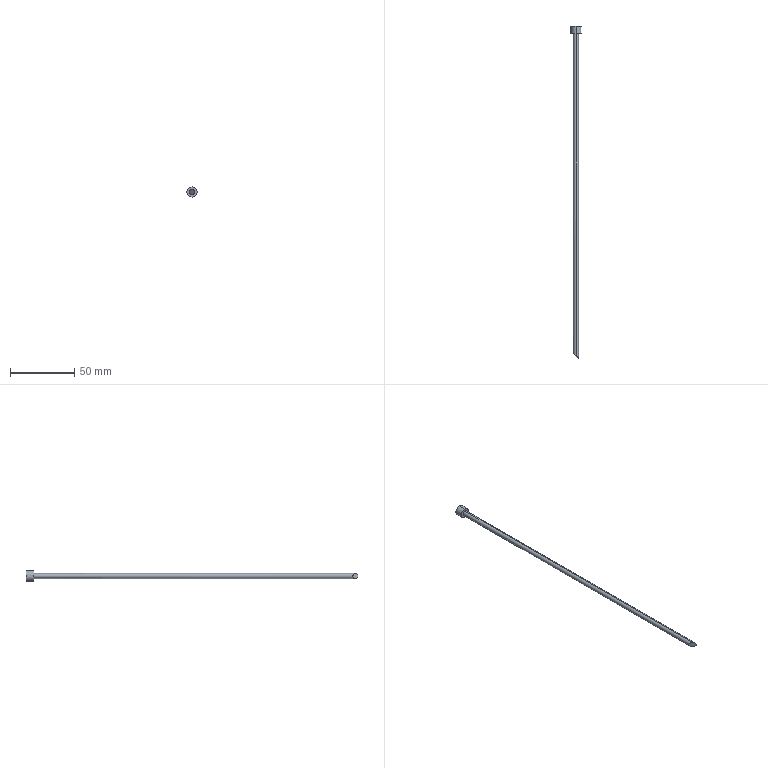Part | STEP file | 1 solid | 7 faces | box 8 x 258.534 x 8 mm | volume 3450 mm3 | cylinder 4 | plane 3 | commonest cylinder face diameters 4 x2 8 x2
STEP:
#1=CARTESIAN_POINT('',(0.,0.,0.));
#2=DIRECTION('',(0.,0.,1.));
#3=DIRECTION('',(1.,0.,0.));
#4=AXIS2_PLACEMENT_3D('',#1,#2,#3);
#5=CARTESIAN_POINT('',(-8.338,290.5,79.529));
#6=VERTEX_POINT('',#5);
#7=CARTESIAN_POINT('',(-8.338,290.5,87.529));
#8=VERTEX_POINT('',#7);
#9=CARTESIAN_POINT('',(-8.338,290.5,83.529));
#10=DIRECTION('',(0.,-1.,0.));
#11=DIRECTION('',(0.,0.,-1.));
#12=AXIS2_PLACEMENT_3D('',#9,#10,#11);
#13=CIRCLE('',#12,4.);
#14=CARTESIAN_POINT('',(-8.338,290.5,83.529));
#15=DIRECTION('',(0.,-1.,0.));
#16=DIRECTION('',(0.,0.,-1.));
#17=AXIS2_PLACEMENT_3D('',#14,#15,#16);
#18=CYLINDRICAL_SURFACE('',#17,4.);
#19=CARTESIAN_POINT('',(0.,0.));
#20=DIRECTION('',(1.,0.));
#21=VECTOR('',#20,1.);
#22=LINE('',#19,#21);
#23=(GEOMETRIC_REPRESENTATION_CONTEXT(2)PARAMETRIC_REPRESENTATION_CONTEXT()REPRESENTATION_CONTEXT('',''));
#24=DEFINITIONAL_REPRESENTATION('',(#22),#23);
#25=PCURVE('',#18,#24);
#26=CARTESIAN_POINT('',(-72.862,290.5,110.196));
#27=DIRECTION('',(0.,-1.,0.));
#28=DIRECTION('',(0.,0.,-1.));
#29=AXIS2_PLACEMENT_3D('',#26,#27,#28);
#30=PLANE('',#29);
#31=CARTESIAN_POINT('',(26.667,64.524));
#32=DIRECTION('',(1.,0.));
#33=AXIS2_PLACEMENT_2D('',#31,#32);
#34=CIRCLE('',#33,4.);
#35=(GEOMETRIC_REPRESENTATION_CONTEXT(2)PARAMETRIC_REPRESENTATION_CONTEXT()REPRESENTATION_CONTEXT('',''));
#36=DEFINITIONAL_REPRESENTATION('',(#34),#35);
#37=PCURVE('',#30,#36);
#38=SURFACE_CURVE('',#13,(#25,#37),.PCURVE_S1.);
#39=EDGE_CURVE('',#6,#8,#38,.T.);
#40=ORIENTED_EDGE('',*,*,#39,.T.);
#41=CARTESIAN_POINT('',(-8.338,284.5,87.529));
#42=VERTEX_POINT('',#41);
#43=CARTESIAN_POINT('',(-8.338,290.5,87.529));
#44=DIRECTION('',(0.,-1.,0.));
#45=VECTOR('',#44,1.);
#46=LINE('',#43,#45);
#47=CARTESIAN_POINT('',(3.142,0.));
#48=DIRECTION('',(0.,1.));
#49=VECTOR('',#48,1.);
#50=LINE('',#47,#49);
#51=(GEOMETRIC_REPRESENTATION_CONTEXT(2)PARAMETRIC_REPRESENTATION_CONTEXT()REPRESENTATION_CONTEXT('',''));
#52=DEFINITIONAL_REPRESENTATION('',(#50),#51);
#53=PCURVE('',#18,#52);
#54=CARTESIAN_POINT('',(-8.338,290.5,83.529));
#55=DIRECTION('',(0.,-1.,0.));
#56=DIRECTION('',(0.,0.,-1.));
#57=AXIS2_PLACEMENT_3D('',#54,#55,#56);
#58=CYLINDRICAL_SURFACE('',#57,4.);
#59=CARTESIAN_POINT('',(3.142,0.));
#60=DIRECTION('',(0.,1.));
#61=VECTOR('',#60,1.);
#62=LINE('',#59,#61);
#63=(GEOMETRIC_REPRESENTATION_CONTEXT(2)PARAMETRIC_REPRESENTATION_CONTEXT()REPRESENTATION_CONTEXT('',''));
#64=DEFINITIONAL_REPRESENTATION('',(#62),#63);
#65=PCURVE('',#58,#64);
#66=SURFACE_CURVE('',#46,(#53,#65),.PCURVE_S1.);
#67=EDGE_CURVE('',#8,#42,#66,.T.);
#68=ORIENTED_EDGE('',*,*,#67,.T.);
#69=CARTESIAN_POINT('',(-8.338,284.5,79.529));
#70=VERTEX_POINT('',#69);
#71=CARTESIAN_POINT('',(-8.338,284.5,83.529));
#72=DIRECTION('',(0.,1.,0.));
#73=DIRECTION('',(0.,0.,1.));
#74=AXIS2_PLACEMENT_3D('',#71,#72,#73);
#75=CIRCLE('',#74,4.);
#76=CARTESIAN_POINT('',(3.142,6.));
#77=DIRECTION('',(-1.,0.));
#78=VECTOR('',#77,1.);
#79=LINE('',#76,#78);
#80=(GEOMETRIC_REPRESENTATION_CONTEXT(2)PARAMETRIC_REPRESENTATION_CONTEXT()REPRESENTATION_CONTEXT('',''));
#81=DEFINITIONAL_REPRESENTATION('',(#79),#80);
#82=PCURVE('',#18,#81);
#83=CARTESIAN_POINT('',(-8.338,284.5,83.529));
#84=DIRECTION('',(0.,-1.,0.));
#85=DIRECTION('',(0.,0.,-1.));
#86=AXIS2_PLACEMENT_3D('',#83,#84,#85);
#87=PLANE('',#86);
#88=CARTESIAN_POINT('',(-4.,0.));
#89=CARTESIAN_POINT('',(-4.,6.928));
#90=CARTESIAN_POINT('',(2.,3.464));
#91=CARTESIAN_POINT('',(8.,0.));
#92=CARTESIAN_POINT('',(2.,-3.464));
#93=CARTESIAN_POINT('',(-4.,-6.928));
#94=CARTESIAN_POINT('',(-4.,0.));
#95=(BOUNDED_CURVE()B_SPLINE_CURVE(2,(#88,#89,#90,#91,#92,#93,#94),.UNSPECIFIED.,.T.,.F.)B_SPLINE_CURVE_WITH_KNOTS((1,2,2,2,2,1),(-2.094,0.,2.094,4.189,6.283,8.378),.UNSPECIFIED.)CURVE()GEOMETRIC_REPRESENTATION_ITEM()RATIONAL_B_SPLINE_CURVE((1.,0.5,1.,0.5,1.,0.5,1.))REPRESENTATION_ITEM(''));
#96=(GEOMETRIC_REPRESENTATION_CONTEXT(2)PARAMETRIC_REPRESENTATION_CONTEXT()REPRESENTATION_CONTEXT('',''));
#97=DEFINITIONAL_REPRESENTATION('',(#95),#96);
#98=PCURVE('',#87,#97);
#99=SURFACE_CURVE('',#75,(#82,#98),.PCURVE_S1.);
#100=EDGE_CURVE('',#42,#70,#99,.T.);
#101=ORIENTED_EDGE('',*,*,#100,.T.);
#102=CARTESIAN_POINT('',(-8.338,290.5,79.529));
#103=DIRECTION('',(0.,-1.,0.));
#104=VECTOR('',#103,1.);
#105=LINE('',#102,#104);
#106=CARTESIAN_POINT('',(0.,0.));
#107=DIRECTION('',(0.,1.));
#108=VECTOR('',#107,1.);
#109=LINE('',#106,#108);
#110=(GEOMETRIC_REPRESENTATION_CONTEXT(2)PARAMETRIC_REPRESENTATION_CONTEXT()REPRESENTATION_CONTEXT('',''));
#111=DEFINITIONAL_REPRESENTATION('',(#109),#110);
#112=PCURVE('',#18,#111);
#113=CARTESIAN_POINT('',(6.283,0.));
#114=DIRECTION('',(0.,1.));
#115=VECTOR('',#114,1.);
#116=LINE('',#113,#115);
#117=(GEOMETRIC_REPRESENTATION_CONTEXT(2)PARAMETRIC_REPRESENTATION_CONTEXT()REPRESENTATION_CONTEXT('',''));
#118=DEFINITIONAL_REPRESENTATION('',(#116),#117);
#119=PCURVE('',#58,#118);
#120=SURFACE_CURVE('',#105,(#112,#119),.PCURVE_S1.);
#121=EDGE_CURVE('',#6,#70,#120,.T.);
#122=ORIENTED_EDGE('',*,*,#121,.F.);
#123=EDGE_LOOP('',(#40,#68,#101,#122));
#124=FACE_BOUND('',#123,.T.);
#125=ADVANCED_FACE('',(#124),#18,.T.);
#126=CARTESIAN_POINT('',(-8.338,284.5,85.529));
#127=VERTEX_POINT('',#126);
#128=CARTESIAN_POINT('',(-8.338,284.5,81.529));
#129=VERTEX_POINT('',#128);
#130=CARTESIAN_POINT('',(-8.338,284.5,83.529));
#131=DIRECTION('',(0.,1.,0.));
#132=DIRECTION('',(0.,0.,-1.));
#133=AXIS2_PLACEMENT_3D('',#130,#131,#132);
#134=CIRCLE('',#133,2.);
#135=CARTESIAN_POINT('',(-8.338,220.5,83.529));
#136=DIRECTION('',(0.,-1.,0.));
#137=DIRECTION('',(0.,0.,-1.));
#138=AXIS2_PLACEMENT_3D('',#135,#136,#137);
#139=CYLINDRICAL_SURFACE('',#138,2.);
#140=CARTESIAN_POINT('',(6.283,-64.));
#141=DIRECTION('',(-1.,0.));
#142=VECTOR('',#141,1.);
#143=LINE('',#140,#142);
#144=(GEOMETRIC_REPRESENTATION_CONTEXT(2)PARAMETRIC_REPRESENTATION_CONTEXT()REPRESENTATION_CONTEXT('',''));
#145=DEFINITIONAL_REPRESENTATION('',(#143),#144);
#146=PCURVE('',#139,#145);
#147=CARTESIAN_POINT('',(2.,0.));
#148=CARTESIAN_POINT('',(2.,-3.464));
#149=CARTESIAN_POINT('',(-1.,-1.732));
#150=CARTESIAN_POINT('',(-4.,0.));
#151=CARTESIAN_POINT('',(-1.,1.732));
#152=CARTESIAN_POINT('',(2.,3.464));
#153=CARTESIAN_POINT('',(2.,0.));
#154=(BOUNDED_CURVE()B_SPLINE_CURVE(2,(#147,#148,#149,#150,#151,#152,#153),.UNSPECIFIED.,.T.,.F.)B_SPLINE_CURVE_WITH_KNOTS((1,2,2,2,2,1),(-2.094,0.,2.094,4.189,6.283,8.378),.UNSPECIFIED.)CURVE()GEOMETRIC_REPRESENTATION_ITEM()RATIONAL_B_SPLINE_CURVE((1.,0.5,1.,0.5,1.,0.5,1.))REPRESENTATION_ITEM(''));
#155=(GEOMETRIC_REPRESENTATION_CONTEXT(2)PARAMETRIC_REPRESENTATION_CONTEXT()REPRESENTATION_CONTEXT('',''));
#156=DEFINITIONAL_REPRESENTATION('',(#154),#155);
#157=PCURVE('',#87,#156);
#158=SURFACE_CURVE('',#134,(#146,#157),.PCURVE_S1.);
#159=EDGE_CURVE('',#127,#129,#158,.T.);
#160=ORIENTED_EDGE('',*,*,#159,.F.);
#161=CARTESIAN_POINT('',(-8.338,33.966,85.529));
#162=VERTEX_POINT('',#161);
#163=CARTESIAN_POINT('',(-8.338,220.5,85.529));
#164=DIRECTION('',(0.,-1.,0.));
#165=VECTOR('',#164,1.);
#166=LINE('',#163,#165);
#167=CARTESIAN_POINT('',(3.142,0.));
#168=DIRECTION('',(0.,1.));
#169=VECTOR('',#168,1.);
#170=LINE('',#167,#169);
#171=(GEOMETRIC_REPRESENTATION_CONTEXT(2)PARAMETRIC_REPRESENTATION_CONTEXT()REPRESENTATION_CONTEXT('',''));
#172=DEFINITIONAL_REPRESENTATION('',(#170),#171);
#173=PCURVE('',#139,#172);
#174=CARTESIAN_POINT('',(-8.338,220.5,83.529));
#175=DIRECTION('',(0.,-1.,0.));
#176=DIRECTION('',(0.,0.,-1.));
#177=AXIS2_PLACEMENT_3D('',#174,#175,#176);
#178=CYLINDRICAL_SURFACE('',#177,2.);
#179=CARTESIAN_POINT('',(3.142,0.));
#180=DIRECTION('',(0.,1.));
#181=VECTOR('',#180,1.);
#182=LINE('',#179,#181);
#183=(GEOMETRIC_REPRESENTATION_CONTEXT(2)PARAMETRIC_REPRESENTATION_CONTEXT()REPRESENTATION_CONTEXT('',''));
#184=DEFINITIONAL_REPRESENTATION('',(#182),#183);
#185=PCURVE('',#178,#184);
#186=SURFACE_CURVE('',#166,(#173,#185),.PCURVE_S1.);
#187=EDGE_CURVE('',#127,#162,#186,.T.);
#188=ORIENTED_EDGE('',*,*,#187,.T.);
#189=CARTESIAN_POINT('',(-8.338,33.966,81.529));
#190=VERTEX_POINT('',#189);
#191=CARTESIAN_POINT('',(-8.338,33.966,85.529));
#192=CARTESIAN_POINT('',(-4.338,29.966,85.529));
#193=CARTESIAN_POINT('',(-4.338,29.966,81.529));
#194=CARTESIAN_POINT('',(-8.338,33.966,81.529));
#195=(BOUNDED_CURVE()B_SPLINE_CURVE(3,(#191,#192,#193,#194),.UNSPECIFIED.,.F.,.F.)B_SPLINE_CURVE_WITH_KNOTS((4,4),(4.712,7.854),.PIECEWISE_BEZIER_KNOTS.)CURVE()GEOMETRIC_REPRESENTATION_ITEM()RATIONAL_B_SPLINE_CURVE((1.,0.3333,0.3333,1.))REPRESENTATION_ITEM(''));
#196=CARTESIAN_POINT('',(3.142,186.534));
#197=CARTESIAN_POINT('',(3.111,186.594));
#198=CARTESIAN_POINT('',(3.048,186.721));
#199=CARTESIAN_POINT('',(2.944,186.928));
#200=CARTESIAN_POINT('',(2.83,187.148));
#201=CARTESIAN_POINT('',(2.706,187.38));
#202=CARTESIAN_POINT('',(2.571,187.617));
#203=CARTESIAN_POINT('',(2.426,187.851));
#204=CARTESIAN_POINT('',(2.27,188.071));
#205=CARTESIAN_POINT('',(2.105,188.264));
#206=CARTESIAN_POINT('',(1.931,188.415));
#207=CARTESIAN_POINT('',(1.753,188.512));
#208=CARTESIAN_POINT('',(1.571,188.545));
#209=CARTESIAN_POINT('',(1.389,188.512));
#210=CARTESIAN_POINT('',(1.21,188.415));
#211=CARTESIAN_POINT('',(1.037,188.264));
#212=CARTESIAN_POINT('',(0.8717,188.071));
#213=CARTESIAN_POINT('',(0.7158,187.851));
#214=CARTESIAN_POINT('',(0.5703,187.617));
#215=CARTESIAN_POINT('',(0.4356,187.38));
#216=CARTESIAN_POINT('',(0.3115,187.148));
#217=CARTESIAN_POINT('',(0.1977,186.928));
#218=CARTESIAN_POINT('',(0.09367,186.721));
#219=CARTESIAN_POINT('',(0.0303,186.594));
#220=CARTESIAN_POINT('',(0.,186.534));
#221=B_SPLINE_CURVE_WITH_KNOTS('',3,(#196,#197,#198,#199,#200,#201,#202,#203,#204,#205,#206,#207,#208,#209,#210,#211,#212,#213,#214,#215,#216,#217,#218,#219,#220),.UNSPECIFIED.,.F.,.F.,(4,1,1,1,1,1,1,1,1,1,1,1,1,1,1,1,1,1,1,1,1,1,4),(4.712,4.855,4.998,5.141,5.284,5.426,5.569,5.712,5.855,5.998,6.14,6.283,6.426,6.569,6.712,6.854,6.997,7.14,7.283,7.426,7.568,7.711,7.854),.QUASI_UNIFORM_KNOTS.);
#222=(GEOMETRIC_REPRESENTATION_CONTEXT(2)PARAMETRIC_REPRESENTATION_CONTEXT()REPRESENTATION_CONTEXT('',''));
#223=DEFINITIONAL_REPRESENTATION('',(#221),#222);
#224=PCURVE('',#139,#223);
#225=CARTESIAN_POINT('',(-6.03,31.657,95.475));
#226=DIRECTION('',(-0.7071,-0.7071,0.));
#227=DIRECTION('',(0.7071,-0.7071,0.));
#228=AXIS2_PLACEMENT_3D('',#225,#226,#227);
#229=PLANE('',#228);
#230=CARTESIAN_POINT('',(-3.265,-9.946));
#231=CARTESIAN_POINT('',(2.392,-9.946));
#232=CARTESIAN_POINT('',(2.392,-13.946));
#233=CARTESIAN_POINT('',(-3.265,-13.946));
#234=(BOUNDED_CURVE()B_SPLINE_CURVE(3,(#230,#231,#232,#233),.UNSPECIFIED.,.F.,.F.)B_SPLINE_CURVE_WITH_KNOTS((4,4),(4.712,7.854),.PIECEWISE_BEZIER_KNOTS.)CURVE()GEOMETRIC_REPRESENTATION_ITEM()RATIONAL_B_SPLINE_CURVE((1.,0.3333,0.3333,1.))REPRESENTATION_ITEM(''));
#235=(GEOMETRIC_REPRESENTATION_CONTEXT(2)PARAMETRIC_REPRESENTATION_CONTEXT()REPRESENTATION_CONTEXT('',''));
#236=DEFINITIONAL_REPRESENTATION('',(#234),#235);
#237=PCURVE('',#229,#236);
#238=SURFACE_CURVE('',#195,(#224,#237),.PCURVE_S1.);
#239=EDGE_CURVE('',#162,#190,#238,.T.);
#240=ORIENTED_EDGE('',*,*,#239,.T.);
#241=CARTESIAN_POINT('',(-8.338,220.5,81.529));
#242=DIRECTION('',(0.,-1.,0.));
#243=VECTOR('',#242,1.);
#244=LINE('',#241,#243);
#245=CARTESIAN_POINT('',(0.,0.));
#246=DIRECTION('',(0.,1.));
#247=VECTOR('',#246,1.);
#248=LINE('',#245,#247);
#249=(GEOMETRIC_REPRESENTATION_CONTEXT(2)PARAMETRIC_REPRESENTATION_CONTEXT()REPRESENTATION_CONTEXT('',''));
#250=DEFINITIONAL_REPRESENTATION('',(#248),#249);
#251=PCURVE('',#139,#250);
#252=CARTESIAN_POINT('',(6.283,0.));
#253=DIRECTION('',(0.,1.));
#254=VECTOR('',#253,1.);
#255=LINE('',#252,#254);
#256=(GEOMETRIC_REPRESENTATION_CONTEXT(2)PARAMETRIC_REPRESENTATION_CONTEXT()REPRESENTATION_CONTEXT('',''));
#257=DEFINITIONAL_REPRESENTATION('',(#255),#256);
#258=PCURVE('',#178,#257);
#259=SURFACE_CURVE('',#244,(#251,#258),.PCURVE_S1.);
#260=EDGE_CURVE('',#129,#190,#259,.T.);
#261=ORIENTED_EDGE('',*,*,#260,.F.);
#262=EDGE_LOOP('',(#160,#188,#240,#261));
#263=FACE_BOUND('',#262,.T.);
#264=ADVANCED_FACE('',(#263),#139,.T.);
#265=ORIENTED_EDGE('',*,*,#187,.F.);
#266=CARTESIAN_POINT('',(-8.338,284.5,83.529));
#267=DIRECTION('',(0.,1.,0.));
#268=DIRECTION('',(0.,0.,-1.));
#269=AXIS2_PLACEMENT_3D('',#266,#267,#268);
#270=CIRCLE('',#269,2.);
#271=CARTESIAN_POINT('',(6.283,-64.));
#272=DIRECTION('',(-1.,0.));
#273=VECTOR('',#272,1.);
#274=LINE('',#271,#273);
#275=(GEOMETRIC_REPRESENTATION_CONTEXT(2)PARAMETRIC_REPRESENTATION_CONTEXT()REPRESENTATION_CONTEXT('',''));
#276=DEFINITIONAL_REPRESENTATION('',(#274),#275);
#277=PCURVE('',#178,#276);
#278=CARTESIAN_POINT('',(2.,0.));
#279=CARTESIAN_POINT('',(2.,-3.464));
#280=CARTESIAN_POINT('',(-1.,-1.732));
#281=CARTESIAN_POINT('',(-4.,0.));
#282=CARTESIAN_POINT('',(-1.,1.732));
#283=CARTESIAN_POINT('',(2.,3.464));
#284=CARTESIAN_POINT('',(2.,0.));
#285=(BOUNDED_CURVE()B_SPLINE_CURVE(2,(#278,#279,#280,#281,#282,#283,#284),.UNSPECIFIED.,.T.,.F.)B_SPLINE_CURVE_WITH_KNOTS((1,2,2,2,2,1),(-2.094,0.,2.094,4.189,6.283,8.378),.UNSPECIFIED.)CURVE()GEOMETRIC_REPRESENTATION_ITEM()RATIONAL_B_SPLINE_CURVE((1.,0.5,1.,0.5,1.,0.5,1.))REPRESENTATION_ITEM(''));
#286=(GEOMETRIC_REPRESENTATION_CONTEXT(2)PARAMETRIC_REPRESENTATION_CONTEXT()REPRESENTATION_CONTEXT('',''));
#287=DEFINITIONAL_REPRESENTATION('',(#285),#286);
#288=PCURVE('',#87,#287);
#289=SURFACE_CURVE('',#270,(#277,#288),.PCURVE_S1.);
#290=EDGE_CURVE('',#129,#127,#289,.T.);
#291=ORIENTED_EDGE('',*,*,#290,.F.);
#292=ORIENTED_EDGE('',*,*,#260,.T.);
#293=CARTESIAN_POINT('',(-8.338,33.966,81.529));
#294=CARTESIAN_POINT('',(-12.338,37.966,81.529));
#295=CARTESIAN_POINT('',(-12.338,37.966,85.529));
#296=CARTESIAN_POINT('',(-8.338,33.966,85.529));
#297=(BOUNDED_CURVE()B_SPLINE_CURVE(3,(#293,#294,#295,#296),.UNSPECIFIED.,.F.,.F.)B_SPLINE_CURVE_WITH_KNOTS((4,4),(1.571,4.712),.PIECEWISE_BEZIER_KNOTS.)CURVE()GEOMETRIC_REPRESENTATION_ITEM()RATIONAL_B_SPLINE_CURVE((1.,0.3333,0.3333,1.))REPRESENTATION_ITEM(''));
#298=CARTESIAN_POINT('',(6.283,186.534));
#299=CARTESIAN_POINT('',(6.253,186.474));
#300=CARTESIAN_POINT('',(6.19,186.347));
#301=CARTESIAN_POINT('',(6.085,186.14));
#302=CARTESIAN_POINT('',(5.972,185.92));
#303=CARTESIAN_POINT('',(5.848,185.688));
#304=CARTESIAN_POINT('',(5.713,185.451));
#305=CARTESIAN_POINT('',(5.567,185.217));
#306=CARTESIAN_POINT('',(5.412,184.997));
#307=CARTESIAN_POINT('',(5.246,184.804));
#308=CARTESIAN_POINT('',(5.073,184.653));
#309=CARTESIAN_POINT('',(4.894,184.556));
#310=CARTESIAN_POINT('',(4.712,184.523));
#311=CARTESIAN_POINT('',(4.531,184.556));
#312=CARTESIAN_POINT('',(4.352,184.653));
#313=CARTESIAN_POINT('',(4.179,184.804));
#314=CARTESIAN_POINT('',(4.013,184.997));
#315=CARTESIAN_POINT('',(3.857,185.217));
#316=CARTESIAN_POINT('',(3.712,185.451));
#317=CARTESIAN_POINT('',(3.577,185.688));
#318=CARTESIAN_POINT('',(3.453,185.92));
#319=CARTESIAN_POINT('',(3.339,186.14));
#320=CARTESIAN_POINT('',(3.235,186.347));
#321=CARTESIAN_POINT('',(3.172,186.474));
#322=CARTESIAN_POINT('',(3.142,186.534));
#323=B_SPLINE_CURVE_WITH_KNOTS('',3,(#298,#299,#300,#301,#302,#303,#304,#305,#306,#307,#308,#309,#310,#311,#312,#313,#314,#315,#316,#317,#318,#319,#320,#321,#322),.UNSPECIFIED.,.F.,.F.,(4,1,1,1,1,1,1,1,1,1,1,1,1,1,1,1,1,1,1,1,1,1,4),(1.571,1.714,1.856,1.999,2.142,2.285,2.428,2.57,2.713,2.856,2.999,3.142,3.284,3.427,3.57,3.713,3.856,3.998,4.141,4.284,4.427,4.57,4.712),.QUASI_UNIFORM_KNOTS.);
#324=(GEOMETRIC_REPRESENTATION_CONTEXT(2)PARAMETRIC_REPRESENTATION_CONTEXT()REPRESENTATION_CONTEXT('',''));
#325=DEFINITIONAL_REPRESENTATION('',(#323),#324);
#326=PCURVE('',#178,#325);
#327=CARTESIAN_POINT('',(-3.265,-13.946));
#328=CARTESIAN_POINT('',(-8.922,-13.946));
#329=CARTESIAN_POINT('',(-8.922,-9.946));
#330=CARTESIAN_POINT('',(-3.265,-9.946));
#331=(BOUNDED_CURVE()B_SPLINE_CURVE(3,(#327,#328,#329,#330),.UNSPECIFIED.,.F.,.F.)B_SPLINE_CURVE_WITH_KNOTS((4,4),(1.571,4.712),.PIECEWISE_BEZIER_KNOTS.)CURVE()GEOMETRIC_REPRESENTATION_ITEM()RATIONAL_B_SPLINE_CURVE((1.,0.3333,0.3333,1.))REPRESENTATION_ITEM(''));
#332=(GEOMETRIC_REPRESENTATION_CONTEXT(2)PARAMETRIC_REPRESENTATION_CONTEXT()REPRESENTATION_CONTEXT('',''));
#333=DEFINITIONAL_REPRESENTATION('',(#331),#332);
#334=PCURVE('',#229,#333);
#335=SURFACE_CURVE('',#297,(#326,#334),.PCURVE_S1.);
#336=EDGE_CURVE('',#190,#162,#335,.T.);
#337=ORIENTED_EDGE('',*,*,#336,.T.);
#338=EDGE_LOOP('',(#265,#291,#292,#337));
#339=FACE_BOUND('',#338,.T.);
#340=ADVANCED_FACE('',(#339),#178,.T.);
#341=ORIENTED_EDGE('',*,*,#336,.F.);
#342=ORIENTED_EDGE('',*,*,#239,.F.);
#343=EDGE_LOOP('',(#341,#342));
#344=FACE_BOUND('',#343,.T.);
#345=ADVANCED_FACE('',(#344),#229,.T.);
#346=ORIENTED_EDGE('',*,*,#290,.T.);
#347=ORIENTED_EDGE('',*,*,#159,.T.);
#348=EDGE_LOOP('',(#346,#347));
#349=FACE_BOUND('',#348,.T.);
#350=CARTESIAN_POINT('',(-8.338,284.5,83.529));
#351=DIRECTION('',(0.,1.,0.));
#352=DIRECTION('',(0.,0.,1.));
#353=AXIS2_PLACEMENT_3D('',#350,#351,#352);
#354=CIRCLE('',#353,4.);
#355=CARTESIAN_POINT('',(-4.,0.));
#356=CARTESIAN_POINT('',(-4.,6.928));
#357=CARTESIAN_POINT('',(2.,3.464));
#358=CARTESIAN_POINT('',(8.,0.));
#359=CARTESIAN_POINT('',(2.,-3.464));
#360=CARTESIAN_POINT('',(-4.,-6.928));
#361=CARTESIAN_POINT('',(-4.,0.));
#362=(BOUNDED_CURVE()B_SPLINE_CURVE(2,(#355,#356,#357,#358,#359,#360,#361),.UNSPECIFIED.,.T.,.F.)B_SPLINE_CURVE_WITH_KNOTS((1,2,2,2,2,1),(-2.094,0.,2.094,4.189,6.283,8.378),.UNSPECIFIED.)CURVE()GEOMETRIC_REPRESENTATION_ITEM()RATIONAL_B_SPLINE_CURVE((1.,0.5,1.,0.5,1.,0.5,1.))REPRESENTATION_ITEM(''));
#363=(GEOMETRIC_REPRESENTATION_CONTEXT(2)PARAMETRIC_REPRESENTATION_CONTEXT()REPRESENTATION_CONTEXT('',''));
#364=DEFINITIONAL_REPRESENTATION('',(#362),#363);
#365=PCURVE('',#87,#364);
#366=CARTESIAN_POINT('',(9.425,6.));
#367=DIRECTION('',(-1.,0.));
#368=VECTOR('',#367,1.);
#369=LINE('',#366,#368);
#370=(GEOMETRIC_REPRESENTATION_CONTEXT(2)PARAMETRIC_REPRESENTATION_CONTEXT()REPRESENTATION_CONTEXT('',''));
#371=DEFINITIONAL_REPRESENTATION('',(#369),#370);
#372=PCURVE('',#58,#371);
#373=SURFACE_CURVE('',#354,(#365,#372),.PCURVE_S1.);
#374=EDGE_CURVE('',#70,#42,#373,.T.);
#375=ORIENTED_EDGE('',*,*,#374,.F.);
#376=ORIENTED_EDGE('',*,*,#100,.F.);
#377=EDGE_LOOP('',(#375,#376));
#378=FACE_BOUND('',#377,.T.);
#379=ADVANCED_FACE('',(#349,#378),#87,.T.);
#380=ORIENTED_EDGE('',*,*,#67,.F.);
#381=CARTESIAN_POINT('',(-8.338,290.5,83.529));
#382=DIRECTION('',(0.,-1.,0.));
#383=DIRECTION('',(0.,0.,-1.));
#384=AXIS2_PLACEMENT_3D('',#381,#382,#383);
#385=CIRCLE('',#384,4.);
#386=CARTESIAN_POINT('',(0.,0.));
#387=DIRECTION('',(1.,0.));
#388=VECTOR('',#387,1.);
#389=LINE('',#386,#388);
#390=(GEOMETRIC_REPRESENTATION_CONTEXT(2)PARAMETRIC_REPRESENTATION_CONTEXT()REPRESENTATION_CONTEXT('',''));
#391=DEFINITIONAL_REPRESENTATION('',(#389),#390);
#392=PCURVE('',#58,#391);
#393=CARTESIAN_POINT('',(26.667,64.524));
#394=DIRECTION('',(1.,0.));
#395=AXIS2_PLACEMENT_2D('',#393,#394);
#396=CIRCLE('',#395,4.);
#397=(GEOMETRIC_REPRESENTATION_CONTEXT(2)PARAMETRIC_REPRESENTATION_CONTEXT()REPRESENTATION_CONTEXT('',''));
#398=DEFINITIONAL_REPRESENTATION('',(#396),#397);
#399=PCURVE('',#30,#398);
#400=SURFACE_CURVE('',#385,(#392,#399),.PCURVE_S1.);
#401=EDGE_CURVE('',#8,#6,#400,.T.);
#402=ORIENTED_EDGE('',*,*,#401,.T.);
#403=ORIENTED_EDGE('',*,*,#121,.T.);
#404=ORIENTED_EDGE('',*,*,#374,.T.);
#405=EDGE_LOOP('',(#380,#402,#403,#404));
#406=FACE_BOUND('',#405,.T.);
#407=ADVANCED_FACE('',(#406),#58,.T.);
#408=ORIENTED_EDGE('',*,*,#39,.F.);
#409=ORIENTED_EDGE('',*,*,#401,.F.);
#410=EDGE_LOOP('',(#408,#409));
#411=FACE_BOUND('',#410,.T.);
#412=ADVANCED_FACE('',(#411),#30,.F.);
#413=CLOSED_SHELL('',(#125,#264,#340,#345,#379,#407,#412));
#414=MANIFOLD_SOLID_BREP('',#413);
#415=(LENGTH_UNIT()NAMED_UNIT(*)SI_UNIT(.MILLI.,.METRE.));
#416=UNCERTAINTY_MEASURE_WITH_UNIT(LENGTH_MEASURE(0.0000001),#415,'','');
#417=(NAMED_UNIT(*)PLANE_ANGLE_UNIT()SI_UNIT($,.RADIAN.));
#418=(NAMED_UNIT(*)SI_UNIT($,.STERADIAN.)SOLID_ANGLE_UNIT());
#419=(GEOMETRIC_REPRESENTATION_CONTEXT(3)GLOBAL_UNCERTAINTY_ASSIGNED_CONTEXT((#416))GLOBAL_UNIT_ASSIGNED_CONTEXT((#415,#417,#418))REPRESENTATION_CONTEXT('',''));
#420=ADVANCED_BREP_SHAPE_REPRESENTATION('',(#4,#414),#419);